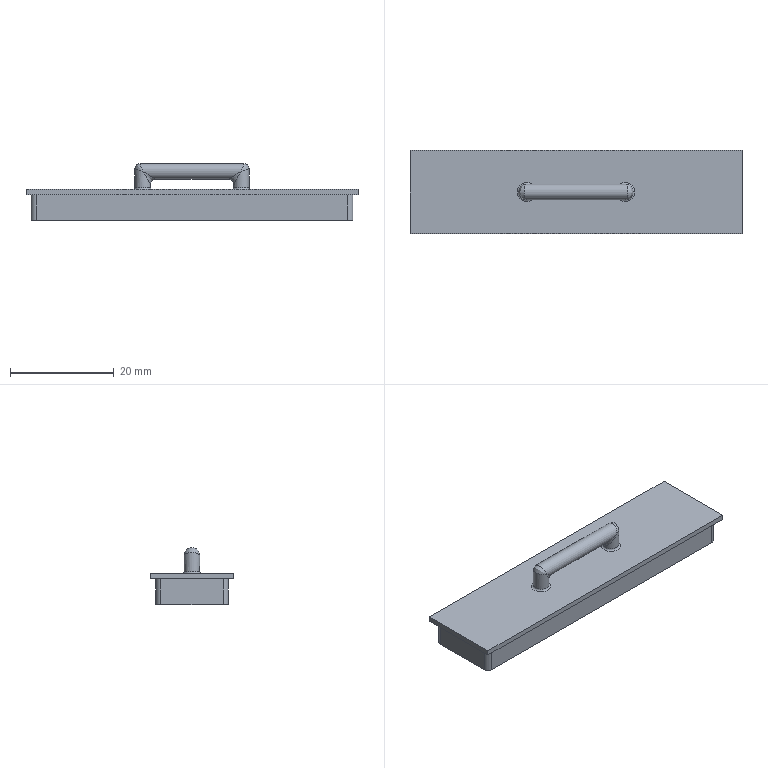Part | STEP file | 1-43.11 | 1 solid | 31 faces | box 64 x 16 x 11 mm | volume 1944 mm3 | plane 16 | cylinder 7 | spline 6 | torus 2 | commonest cylinder face diameters 2 x4 3 x3